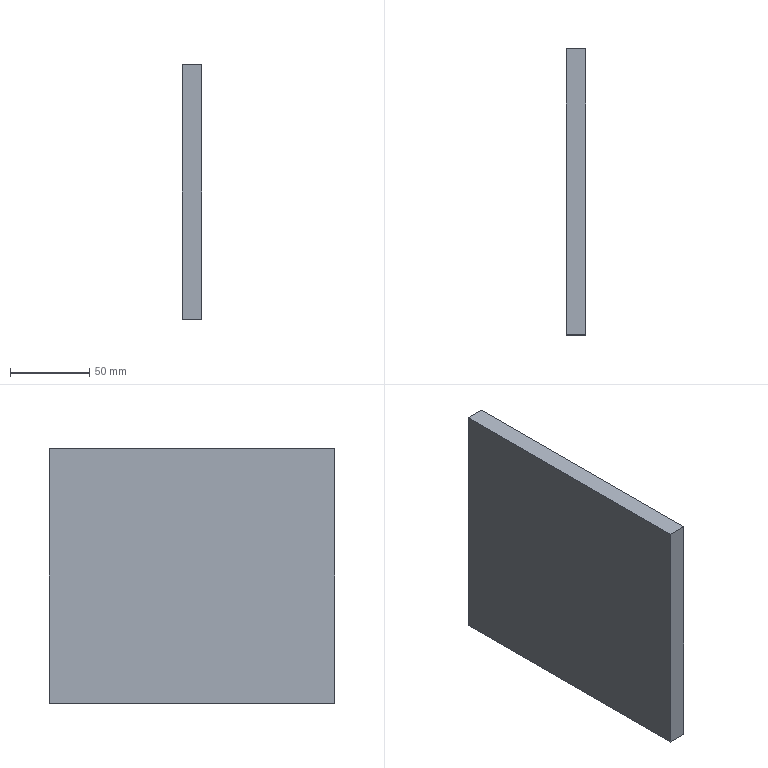Part | STEP file | placa de celeron | 1 solid | 6 faces | box 12 x 180 x 160 mm | volume 345600 mm3 | plane 6
STEP:
#1=CARTESIAN_POINT('',(0.,0.,0.));
#2=DIRECTION('',(0.,0.,1.));
#3=DIRECTION('',(1.,0.,0.));
#4=AXIS2_PLACEMENT_3D('',#1,#2,#3);
#5=CARTESIAN_POINT('',(-82.632,-57.125,-160.));
#6=VERTEX_POINT('',#5);
#7=CARTESIAN_POINT('',(-82.632,-237.125,-160.));
#8=VERTEX_POINT('',#7);
#9=CARTESIAN_POINT('',(-82.632,-57.125,-160.));
#10=DIRECTION('',(0.,-1.,0.));
#11=VECTOR('',#10,1.);
#12=LINE('',#9,#11);
#13=CARTESIAN_POINT('',(-82.632,-57.125,0.));
#14=DIRECTION('',(-1.,0.,0.));
#15=DIRECTION('',(0.,0.,1.));
#16=AXIS2_PLACEMENT_3D('',#13,#14,#15);
#17=PLANE('',#16);
#18=CARTESIAN_POINT('',(-160.,0.));
#19=DIRECTION('',(0.,-1.));
#20=VECTOR('',#19,1.);
#21=LINE('',#18,#20);
#22=(GEOMETRIC_REPRESENTATION_CONTEXT(2)PARAMETRIC_REPRESENTATION_CONTEXT()REPRESENTATION_CONTEXT('',''));
#23=DEFINITIONAL_REPRESENTATION('',(#21),#22);
#24=PCURVE('',#17,#23);
#25=CARTESIAN_POINT('',(-76.632,-147.125,-160.));
#26=DIRECTION('',(0.,0.,1.));
#27=DIRECTION('',(1.,0.,0.));
#28=AXIS2_PLACEMENT_3D('',#25,#26,#27);
#29=PLANE('',#28);
#30=CARTESIAN_POINT('',(-6.,90.));
#31=DIRECTION('',(0.,-1.));
#32=VECTOR('',#31,1.);
#33=LINE('',#30,#32);
#34=(GEOMETRIC_REPRESENTATION_CONTEXT(2)PARAMETRIC_REPRESENTATION_CONTEXT()REPRESENTATION_CONTEXT('',''));
#35=DEFINITIONAL_REPRESENTATION('',(#33),#34);
#36=PCURVE('',#29,#35);
#37=SURFACE_CURVE('',#12,(#24,#36),.PCURVE_S1.);
#38=EDGE_CURVE('',#6,#8,#37,.T.);
#39=ORIENTED_EDGE('',*,*,#38,.T.);
#40=CARTESIAN_POINT('',(-82.632,-237.125,0.));
#41=VERTEX_POINT('',#40);
#42=CARTESIAN_POINT('',(-82.632,-237.125,0.));
#43=DIRECTION('',(0.,0.,-1.));
#44=VECTOR('',#43,1.);
#45=LINE('',#42,#44);
#46=CARTESIAN_POINT('',(0.,-180.));
#47=DIRECTION('',(-1.,0.));
#48=VECTOR('',#47,1.);
#49=LINE('',#46,#48);
#50=(GEOMETRIC_REPRESENTATION_CONTEXT(2)PARAMETRIC_REPRESENTATION_CONTEXT()REPRESENTATION_CONTEXT('',''));
#51=DEFINITIONAL_REPRESENTATION('',(#49),#50);
#52=PCURVE('',#17,#51);
#53=CARTESIAN_POINT('',(-82.632,-237.125,0.));
#54=DIRECTION('',(0.,-1.,0.));
#55=DIRECTION('',(0.,0.,-1.));
#56=AXIS2_PLACEMENT_3D('',#53,#54,#55);
#57=PLANE('',#56);
#58=CARTESIAN_POINT('',(0.,0.));
#59=DIRECTION('',(1.,0.));
#60=VECTOR('',#59,1.);
#61=LINE('',#58,#60);
#62=(GEOMETRIC_REPRESENTATION_CONTEXT(2)PARAMETRIC_REPRESENTATION_CONTEXT()REPRESENTATION_CONTEXT('',''));
#63=DEFINITIONAL_REPRESENTATION('',(#61),#62);
#64=PCURVE('',#57,#63);
#65=SURFACE_CURVE('',#45,(#52,#64),.PCURVE_S1.);
#66=EDGE_CURVE('',#41,#8,#65,.T.);
#67=ORIENTED_EDGE('',*,*,#66,.F.);
#68=CARTESIAN_POINT('',(-82.632,-57.125,0.));
#69=VERTEX_POINT('',#68);
#70=CARTESIAN_POINT('',(-82.632,-237.125,0.));
#71=DIRECTION('',(0.,1.,0.));
#72=VECTOR('',#71,1.);
#73=LINE('',#70,#72);
#74=CARTESIAN_POINT('',(0.,-180.));
#75=DIRECTION('',(0.,1.));
#76=VECTOR('',#75,1.);
#77=LINE('',#74,#76);
#78=(GEOMETRIC_REPRESENTATION_CONTEXT(2)PARAMETRIC_REPRESENTATION_CONTEXT()REPRESENTATION_CONTEXT('',''));
#79=DEFINITIONAL_REPRESENTATION('',(#77),#78);
#80=PCURVE('',#17,#79);
#81=CARTESIAN_POINT('',(-76.632,-147.125,0.));
#82=DIRECTION('',(0.,0.,1.));
#83=DIRECTION('',(1.,0.,0.));
#84=AXIS2_PLACEMENT_3D('',#81,#82,#83);
#85=PLANE('',#84);
#86=CARTESIAN_POINT('',(-6.,-90.));
#87=DIRECTION('',(0.,1.));
#88=VECTOR('',#87,1.);
#89=LINE('',#86,#88);
#90=(GEOMETRIC_REPRESENTATION_CONTEXT(2)PARAMETRIC_REPRESENTATION_CONTEXT()REPRESENTATION_CONTEXT('',''));
#91=DEFINITIONAL_REPRESENTATION('',(#89),#90);
#92=PCURVE('',#85,#91);
#93=SURFACE_CURVE('',#73,(#80,#92),.PCURVE_S1.);
#94=EDGE_CURVE('',#41,#69,#93,.T.);
#95=ORIENTED_EDGE('',*,*,#94,.T.);
#96=CARTESIAN_POINT('',(-82.632,-57.125,0.));
#97=DIRECTION('',(0.,0.,-1.));
#98=VECTOR('',#97,1.);
#99=LINE('',#96,#98);
#100=CARTESIAN_POINT('',(0.,0.));
#101=DIRECTION('',(-1.,0.));
#102=VECTOR('',#101,1.);
#103=LINE('',#100,#102);
#104=(GEOMETRIC_REPRESENTATION_CONTEXT(2)PARAMETRIC_REPRESENTATION_CONTEXT()REPRESENTATION_CONTEXT('',''));
#105=DEFINITIONAL_REPRESENTATION('',(#103),#104);
#106=PCURVE('',#17,#105);
#107=CARTESIAN_POINT('',(-70.632,-57.125,0.));
#108=DIRECTION('',(0.,1.,0.));
#109=DIRECTION('',(0.,0.,1.));
#110=AXIS2_PLACEMENT_3D('',#107,#108,#109);
#111=PLANE('',#110);
#112=CARTESIAN_POINT('',(0.,-12.));
#113=DIRECTION('',(-1.,0.));
#114=VECTOR('',#113,1.);
#115=LINE('',#112,#114);
#116=(GEOMETRIC_REPRESENTATION_CONTEXT(2)PARAMETRIC_REPRESENTATION_CONTEXT()REPRESENTATION_CONTEXT('',''));
#117=DEFINITIONAL_REPRESENTATION('',(#115),#116);
#118=PCURVE('',#111,#117);
#119=SURFACE_CURVE('',#99,(#106,#118),.PCURVE_S1.);
#120=EDGE_CURVE('',#69,#6,#119,.T.);
#121=ORIENTED_EDGE('',*,*,#120,.T.);
#122=EDGE_LOOP('',(#39,#67,#95,#121));
#123=FACE_BOUND('',#122,.T.);
#124=ADVANCED_FACE('',(#123),#17,.T.);
#125=CARTESIAN_POINT('',(-70.632,-237.125,-160.));
#126=VERTEX_POINT('',#125);
#127=CARTESIAN_POINT('',(-82.632,-237.125,-160.));
#128=DIRECTION('',(1.,0.,0.));
#129=VECTOR('',#128,1.);
#130=LINE('',#127,#129);
#131=CARTESIAN_POINT('',(160.,0.));
#132=DIRECTION('',(0.,1.));
#133=VECTOR('',#132,1.);
#134=LINE('',#131,#133);
#135=(GEOMETRIC_REPRESENTATION_CONTEXT(2)PARAMETRIC_REPRESENTATION_CONTEXT()REPRESENTATION_CONTEXT('',''));
#136=DEFINITIONAL_REPRESENTATION('',(#134),#135);
#137=PCURVE('',#57,#136);
#138=CARTESIAN_POINT('',(-6.,-90.));
#139=DIRECTION('',(1.,0.));
#140=VECTOR('',#139,1.);
#141=LINE('',#138,#140);
#142=(GEOMETRIC_REPRESENTATION_CONTEXT(2)PARAMETRIC_REPRESENTATION_CONTEXT()REPRESENTATION_CONTEXT('',''));
#143=DEFINITIONAL_REPRESENTATION('',(#141),#142);
#144=PCURVE('',#29,#143);
#145=SURFACE_CURVE('',#130,(#137,#144),.PCURVE_S1.);
#146=EDGE_CURVE('',#8,#126,#145,.T.);
#147=ORIENTED_EDGE('',*,*,#146,.T.);
#148=CARTESIAN_POINT('',(-70.632,-237.125,0.));
#149=VERTEX_POINT('',#148);
#150=CARTESIAN_POINT('',(-70.632,-237.125,0.));
#151=DIRECTION('',(0.,0.,-1.));
#152=VECTOR('',#151,1.);
#153=LINE('',#150,#152);
#154=CARTESIAN_POINT('',(0.,12.));
#155=DIRECTION('',(1.,0.));
#156=VECTOR('',#155,1.);
#157=LINE('',#154,#156);
#158=(GEOMETRIC_REPRESENTATION_CONTEXT(2)PARAMETRIC_REPRESENTATION_CONTEXT()REPRESENTATION_CONTEXT('',''));
#159=DEFINITIONAL_REPRESENTATION('',(#157),#158);
#160=PCURVE('',#57,#159);
#161=CARTESIAN_POINT('',(-70.632,-237.125,0.));
#162=DIRECTION('',(1.,0.,0.));
#163=DIRECTION('',(0.,0.,-1.));
#164=AXIS2_PLACEMENT_3D('',#161,#162,#163);
#165=PLANE('',#164);
#166=CARTESIAN_POINT('',(0.,0.));
#167=DIRECTION('',(1.,0.));
#168=VECTOR('',#167,1.);
#169=LINE('',#166,#168);
#170=(GEOMETRIC_REPRESENTATION_CONTEXT(2)PARAMETRIC_REPRESENTATION_CONTEXT()REPRESENTATION_CONTEXT('',''));
#171=DEFINITIONAL_REPRESENTATION('',(#169),#170);
#172=PCURVE('',#165,#171);
#173=SURFACE_CURVE('',#153,(#160,#172),.PCURVE_S1.);
#174=EDGE_CURVE('',#149,#126,#173,.T.);
#175=ORIENTED_EDGE('',*,*,#174,.F.);
#176=CARTESIAN_POINT('',(-70.632,-237.125,0.));
#177=DIRECTION('',(-1.,0.,0.));
#178=VECTOR('',#177,1.);
#179=LINE('',#176,#178);
#180=CARTESIAN_POINT('',(0.,12.));
#181=DIRECTION('',(0.,-1.));
#182=VECTOR('',#181,1.);
#183=LINE('',#180,#182);
#184=(GEOMETRIC_REPRESENTATION_CONTEXT(2)PARAMETRIC_REPRESENTATION_CONTEXT()REPRESENTATION_CONTEXT('',''));
#185=DEFINITIONAL_REPRESENTATION('',(#183),#184);
#186=PCURVE('',#57,#185);
#187=CARTESIAN_POINT('',(6.,-90.));
#188=DIRECTION('',(-1.,0.));
#189=VECTOR('',#188,1.);
#190=LINE('',#187,#189);
#191=(GEOMETRIC_REPRESENTATION_CONTEXT(2)PARAMETRIC_REPRESENTATION_CONTEXT()REPRESENTATION_CONTEXT('',''));
#192=DEFINITIONAL_REPRESENTATION('',(#190),#191);
#193=PCURVE('',#85,#192);
#194=SURFACE_CURVE('',#179,(#186,#193),.PCURVE_S1.);
#195=EDGE_CURVE('',#149,#41,#194,.T.);
#196=ORIENTED_EDGE('',*,*,#195,.T.);
#197=ORIENTED_EDGE('',*,*,#66,.T.);
#198=EDGE_LOOP('',(#147,#175,#196,#197));
#199=FACE_BOUND('',#198,.T.);
#200=ADVANCED_FACE('',(#199),#57,.T.);
#201=CARTESIAN_POINT('',(-70.632,-57.125,-160.));
#202=VERTEX_POINT('',#201);
#203=CARTESIAN_POINT('',(-70.632,-237.125,-160.));
#204=DIRECTION('',(0.,1.,0.));
#205=VECTOR('',#204,1.);
#206=LINE('',#203,#205);
#207=CARTESIAN_POINT('',(160.,0.));
#208=DIRECTION('',(0.,1.));
#209=VECTOR('',#208,1.);
#210=LINE('',#207,#209);
#211=(GEOMETRIC_REPRESENTATION_CONTEXT(2)PARAMETRIC_REPRESENTATION_CONTEXT()REPRESENTATION_CONTEXT('',''));
#212=DEFINITIONAL_REPRESENTATION('',(#210),#211);
#213=PCURVE('',#165,#212);
#214=CARTESIAN_POINT('',(6.,-90.));
#215=DIRECTION('',(0.,1.));
#216=VECTOR('',#215,1.);
#217=LINE('',#214,#216);
#218=(GEOMETRIC_REPRESENTATION_CONTEXT(2)PARAMETRIC_REPRESENTATION_CONTEXT()REPRESENTATION_CONTEXT('',''));
#219=DEFINITIONAL_REPRESENTATION('',(#217),#218);
#220=PCURVE('',#29,#219);
#221=SURFACE_CURVE('',#206,(#213,#220),.PCURVE_S1.);
#222=EDGE_CURVE('',#126,#202,#221,.T.);
#223=ORIENTED_EDGE('',*,*,#222,.T.);
#224=CARTESIAN_POINT('',(-70.632,-57.125,0.));
#225=VERTEX_POINT('',#224);
#226=CARTESIAN_POINT('',(-70.632,-57.125,0.));
#227=DIRECTION('',(0.,0.,-1.));
#228=VECTOR('',#227,1.);
#229=LINE('',#226,#228);
#230=CARTESIAN_POINT('',(0.,180.));
#231=DIRECTION('',(1.,0.));
#232=VECTOR('',#231,1.);
#233=LINE('',#230,#232);
#234=(GEOMETRIC_REPRESENTATION_CONTEXT(2)PARAMETRIC_REPRESENTATION_CONTEXT()REPRESENTATION_CONTEXT('',''));
#235=DEFINITIONAL_REPRESENTATION('',(#233),#234);
#236=PCURVE('',#165,#235);
#237=CARTESIAN_POINT('',(0.,0.));
#238=DIRECTION('',(-1.,0.));
#239=VECTOR('',#238,1.);
#240=LINE('',#237,#239);
#241=(GEOMETRIC_REPRESENTATION_CONTEXT(2)PARAMETRIC_REPRESENTATION_CONTEXT()REPRESENTATION_CONTEXT('',''));
#242=DEFINITIONAL_REPRESENTATION('',(#240),#241);
#243=PCURVE('',#111,#242);
#244=SURFACE_CURVE('',#229,(#236,#243),.PCURVE_S1.);
#245=EDGE_CURVE('',#225,#202,#244,.T.);
#246=ORIENTED_EDGE('',*,*,#245,.F.);
#247=CARTESIAN_POINT('',(-70.632,-57.125,0.));
#248=DIRECTION('',(0.,-1.,0.));
#249=VECTOR('',#248,1.);
#250=LINE('',#247,#249);
#251=CARTESIAN_POINT('',(0.,180.));
#252=DIRECTION('',(0.,-1.));
#253=VECTOR('',#252,1.);
#254=LINE('',#251,#253);
#255=(GEOMETRIC_REPRESENTATION_CONTEXT(2)PARAMETRIC_REPRESENTATION_CONTEXT()REPRESENTATION_CONTEXT('',''));
#256=DEFINITIONAL_REPRESENTATION('',(#254),#255);
#257=PCURVE('',#165,#256);
#258=CARTESIAN_POINT('',(6.,90.));
#259=DIRECTION('',(0.,-1.));
#260=VECTOR('',#259,1.);
#261=LINE('',#258,#260);
#262=(GEOMETRIC_REPRESENTATION_CONTEXT(2)PARAMETRIC_REPRESENTATION_CONTEXT()REPRESENTATION_CONTEXT('',''));
#263=DEFINITIONAL_REPRESENTATION('',(#261),#262);
#264=PCURVE('',#85,#263);
#265=SURFACE_CURVE('',#250,(#257,#264),.PCURVE_S1.);
#266=EDGE_CURVE('',#225,#149,#265,.T.);
#267=ORIENTED_EDGE('',*,*,#266,.T.);
#268=ORIENTED_EDGE('',*,*,#174,.T.);
#269=EDGE_LOOP('',(#223,#246,#267,#268));
#270=FACE_BOUND('',#269,.T.);
#271=ADVANCED_FACE('',(#270),#165,.T.);
#272=CARTESIAN_POINT('',(-70.632,-57.125,-160.));
#273=DIRECTION('',(-1.,0.,0.));
#274=VECTOR('',#273,1.);
#275=LINE('',#272,#274);
#276=CARTESIAN_POINT('',(-160.,0.));
#277=DIRECTION('',(0.,-1.));
#278=VECTOR('',#277,1.);
#279=LINE('',#276,#278);
#280=(GEOMETRIC_REPRESENTATION_CONTEXT(2)PARAMETRIC_REPRESENTATION_CONTEXT()REPRESENTATION_CONTEXT('',''));
#281=DEFINITIONAL_REPRESENTATION('',(#279),#280);
#282=PCURVE('',#111,#281);
#283=CARTESIAN_POINT('',(6.,90.));
#284=DIRECTION('',(-1.,0.));
#285=VECTOR('',#284,1.);
#286=LINE('',#283,#285);
#287=(GEOMETRIC_REPRESENTATION_CONTEXT(2)PARAMETRIC_REPRESENTATION_CONTEXT()REPRESENTATION_CONTEXT('',''));
#288=DEFINITIONAL_REPRESENTATION('',(#286),#287);
#289=PCURVE('',#29,#288);
#290=SURFACE_CURVE('',#275,(#282,#289),.PCURVE_S1.);
#291=EDGE_CURVE('',#202,#6,#290,.T.);
#292=ORIENTED_EDGE('',*,*,#291,.T.);
#293=ORIENTED_EDGE('',*,*,#120,.F.);
#294=CARTESIAN_POINT('',(-82.632,-57.125,0.));
#295=DIRECTION('',(1.,0.,0.));
#296=VECTOR('',#295,1.);
#297=LINE('',#294,#296);
#298=CARTESIAN_POINT('',(0.,-12.));
#299=DIRECTION('',(0.,1.));
#300=VECTOR('',#299,1.);
#301=LINE('',#298,#300);
#302=(GEOMETRIC_REPRESENTATION_CONTEXT(2)PARAMETRIC_REPRESENTATION_CONTEXT()REPRESENTATION_CONTEXT('',''));
#303=DEFINITIONAL_REPRESENTATION('',(#301),#302);
#304=PCURVE('',#111,#303);
#305=CARTESIAN_POINT('',(-6.,90.));
#306=DIRECTION('',(1.,0.));
#307=VECTOR('',#306,1.);
#308=LINE('',#305,#307);
#309=(GEOMETRIC_REPRESENTATION_CONTEXT(2)PARAMETRIC_REPRESENTATION_CONTEXT()REPRESENTATION_CONTEXT('',''));
#310=DEFINITIONAL_REPRESENTATION('',(#308),#309);
#311=PCURVE('',#85,#310);
#312=SURFACE_CURVE('',#297,(#304,#311),.PCURVE_S1.);
#313=EDGE_CURVE('',#69,#225,#312,.T.);
#314=ORIENTED_EDGE('',*,*,#313,.T.);
#315=ORIENTED_EDGE('',*,*,#245,.T.);
#316=EDGE_LOOP('',(#292,#293,#314,#315));
#317=FACE_BOUND('',#316,.T.);
#318=ADVANCED_FACE('',(#317),#111,.T.);
#319=ORIENTED_EDGE('',*,*,#313,.F.);
#320=ORIENTED_EDGE('',*,*,#94,.F.);
#321=ORIENTED_EDGE('',*,*,#195,.F.);
#322=ORIENTED_EDGE('',*,*,#266,.F.);
#323=EDGE_LOOP('',(#319,#320,#321,#322));
#324=FACE_BOUND('',#323,.T.);
#325=ADVANCED_FACE('',(#324),#85,.T.);
#326=ORIENTED_EDGE('',*,*,#38,.F.);
#327=ORIENTED_EDGE('',*,*,#291,.F.);
#328=ORIENTED_EDGE('',*,*,#222,.F.);
#329=ORIENTED_EDGE('',*,*,#146,.F.);
#330=EDGE_LOOP('',(#326,#327,#328,#329));
#331=FACE_BOUND('',#330,.T.);
#332=ADVANCED_FACE('',(#331),#29,.F.);
#333=CLOSED_SHELL('',(#124,#200,#271,#318,#325,#332));
#334=MANIFOLD_SOLID_BREP('',#333);
#335=(LENGTH_UNIT()NAMED_UNIT(*)SI_UNIT(.MILLI.,.METRE.));
#336=UNCERTAINTY_MEASURE_WITH_UNIT(LENGTH_MEASURE(0.0000001),#335,'','');
#337=(NAMED_UNIT(*)PLANE_ANGLE_UNIT()SI_UNIT($,.RADIAN.));
#338=(NAMED_UNIT(*)SI_UNIT($,.STERADIAN.)SOLID_ANGLE_UNIT());
#339=(GEOMETRIC_REPRESENTATION_CONTEXT(3)GLOBAL_UNCERTAINTY_ASSIGNED_CONTEXT((#336))GLOBAL_UNIT_ASSIGNED_CONTEXT((#335,#337,#338))REPRESENTATION_CONTEXT('',''));
#340=ADVANCED_BREP_SHAPE_REPRESENTATION('',(#4,#334),#339);